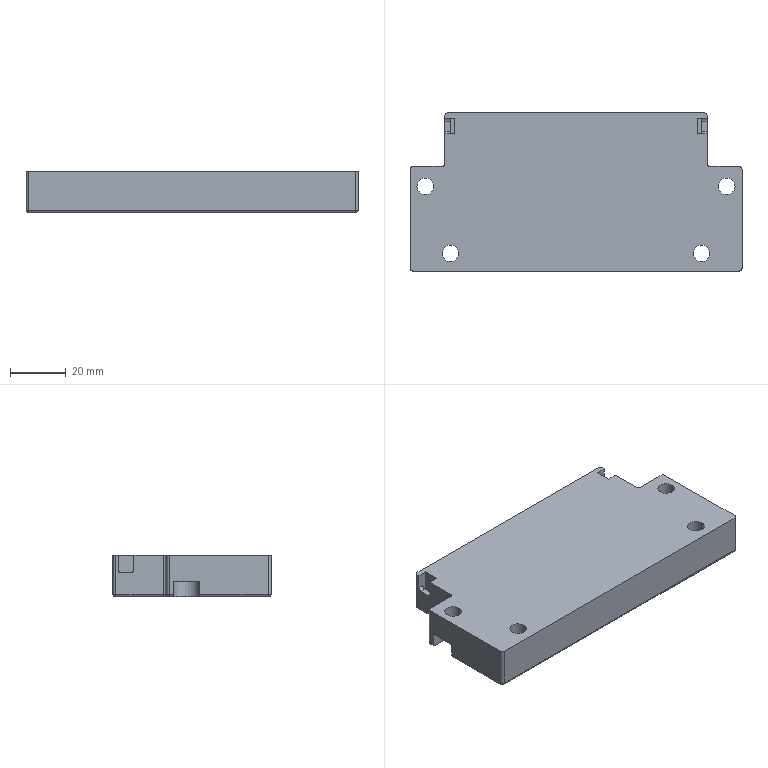Part | STEP file | LES120 front cover^FTH120-PD-direct-drive motor | 1 solid | 559 faces | box 119 x 56.7 x 15 mm | volume 90652 mm3 | plane 336 | spline 174 | cylinder 41 | cone 8 | commonest cylinder face diameters 2 x22 6 x8 2.5 x4 9.2 x4 9.4 x3